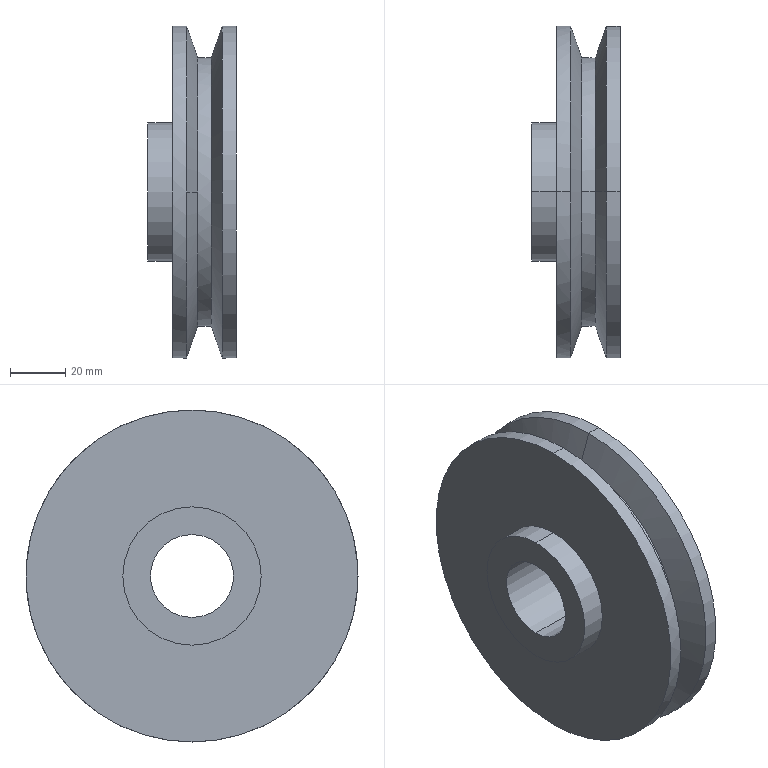Part | SolidWorks | features BaseBody 1, ICE 1 | 1 solid | 17 faces | box 32 x 120 x 120 mm | volume 219683 mm3 | cylinder 10 | cone 4 | plane 3 | commonest cylinder face diameters 120 x4 30 x2 50 x2 97.1 x2
STEP:
#1=CARTESIAN_POINT('',(21.,0.,-15.));
#2=VERTEX_POINT('',#1);
#3=CARTESIAN_POINT('',(21.,0.,15.));
#4=VERTEX_POINT('',#3);
#5=CARTESIAN_POINT('',(21.,0.,0.));
#6=DIRECTION('',(-1.,0.,0.));
#7=DIRECTION('',(0.,0.,1.));
#8=AXIS2_PLACEMENT_3D('',#5,#6,#7);
#9=CIRCLE('',#8,15.);
#10=EDGE_CURVE('',#2,#4,#9,.T.);
#11=ORIENTED_EDGE('',*,*,#10,.F.);
#12=CARTESIAN_POINT('',(-11.,0.,-15.));
#13=VERTEX_POINT('',#12);
#14=CARTESIAN_POINT('',(21.,0.,-15.));
#15=DIRECTION('',(-1.,0.,0.));
#16=VECTOR('',#15,1000.);
#17=LINE('',#14,#16);
#18=EDGE_CURVE('',#2,#13,#17,.T.);
#19=ORIENTED_EDGE('',*,*,#18,.T.);
#20=CARTESIAN_POINT('',(-11.,0.,15.));
#21=VERTEX_POINT('',#20);
#22=CARTESIAN_POINT('',(-11.,0.,0.));
#23=DIRECTION('',(-1.,0.,0.));
#24=DIRECTION('',(0.,0.,1.));
#25=AXIS2_PLACEMENT_3D('',#22,#23,#24);
#26=CIRCLE('',#25,15.);
#27=EDGE_CURVE('',#13,#21,#26,.T.);
#28=ORIENTED_EDGE('',*,*,#27,.T.);
#29=CARTESIAN_POINT('',(21.,0.,15.));
#30=DIRECTION('',(-1.,0.,0.));
#31=VECTOR('',#30,1000.);
#32=LINE('',#29,#31);
#33=EDGE_CURVE('',#4,#21,#32,.T.);
#34=ORIENTED_EDGE('',*,*,#33,.F.);
#35=EDGE_LOOP('',(#11,#19,#28,#34));
#36=FACE_OUTER_BOUND('',#35,.T.);
#37=CARTESIAN_POINT('',(21.,0.,0.));
#38=DIRECTION('',(-1.,0.,0.));
#39=DIRECTION('',(0.,0.,1.));
#40=AXIS2_PLACEMENT_3D('',#37,#38,#39);
#41=CYLINDRICAL_SURFACE('',#40,15.);
#42=ADVANCED_FACE('',(#36),#41,.F.);
#43=CARTESIAN_POINT('',(15.947,0.,-60.));
#44=VERTEX_POINT('',#43);
#45=CARTESIAN_POINT('',(15.947,0.,60.));
#46=VERTEX_POINT('',#45);
#47=CARTESIAN_POINT('',(15.947,0.,0.));
#48=DIRECTION('',(1.,0.,0.));
#49=DIRECTION('',(0.,0.,-1.));
#50=AXIS2_PLACEMENT_3D('',#47,#48,#49);
#51=CIRCLE('',#50,60.);
#52=EDGE_CURVE('',#44,#46,#51,.T.);
#53=ORIENTED_EDGE('',*,*,#52,.T.);
#54=CARTESIAN_POINT('',(21.,0.,60.));
#55=VERTEX_POINT('',#54);
#56=CARTESIAN_POINT('',(0.,0.,60.));
#57=DIRECTION('',(1.,0.,0.));
#58=VECTOR('',#57,1000.);
#59=LINE('',#56,#58);
#60=EDGE_CURVE('',#46,#55,#59,.T.);
#61=ORIENTED_EDGE('',*,*,#60,.T.);
#62=CARTESIAN_POINT('',(21.,0.,-60.));
#63=VERTEX_POINT('',#62);
#64=CARTESIAN_POINT('',(21.,0.,0.));
#65=DIRECTION('',(1.,0.,0.));
#66=DIRECTION('',(0.,0.,-1.));
#67=AXIS2_PLACEMENT_3D('',#64,#65,#66);
#68=CIRCLE('',#67,60.);
#69=EDGE_CURVE('',#63,#55,#68,.T.);
#70=ORIENTED_EDGE('',*,*,#69,.F.);
#71=CARTESIAN_POINT('',(0.,0.,-60.));
#72=DIRECTION('',(1.,0.,0.));
#73=VECTOR('',#72,1000.);
#74=LINE('',#71,#73);
#75=EDGE_CURVE('',#44,#63,#74,.T.);
#76=ORIENTED_EDGE('',*,*,#75,.F.);
#77=EDGE_LOOP('',(#53,#61,#70,#76));
#78=FACE_OUTER_BOUND('',#77,.T.);
#79=CARTESIAN_POINT('',(0.,0.,0.));
#80=DIRECTION('',(1.,0.,0.));
#81=DIRECTION('',(0.,0.,-1.));
#82=AXIS2_PLACEMENT_3D('',#79,#80,#81);
#83=CYLINDRICAL_SURFACE('',#82,60.);
#84=ADVANCED_FACE('',(#78),#83,.T.);
#85=CARTESIAN_POINT('',(12.004,0.,-48.55));
#86=VERTEX_POINT('',#85);
#87=CARTESIAN_POINT('',(12.004,0.,48.55));
#88=VERTEX_POINT('',#87);
#89=CARTESIAN_POINT('',(12.004,0.,0.));
#90=DIRECTION('',(1.,0.,0.));
#91=DIRECTION('',(0.,0.,-1.));
#92=AXIS2_PLACEMENT_3D('',#89,#90,#91);
#93=CIRCLE('',#92,48.55);
#94=EDGE_CURVE('',#86,#88,#93,.T.);
#95=ORIENTED_EDGE('',*,*,#94,.T.);
#96=CARTESIAN_POINT('',(15.947,0.,60.));
#97=DIRECTION('',(0.3256,0.,0.9455));
#98=VECTOR('',#97,1000.);
#99=LINE('',#96,#98);
#100=EDGE_CURVE('',#88,#46,#99,.T.);
#101=ORIENTED_EDGE('',*,*,#100,.T.);
#102=ORIENTED_EDGE('',*,*,#52,.F.);
#103=CARTESIAN_POINT('',(15.947,0.,-60.));
#104=DIRECTION('',(0.3256,0.,-0.9455));
#105=VECTOR('',#104,1000.);
#106=LINE('',#103,#105);
#107=EDGE_CURVE('',#86,#44,#106,.T.);
#108=ORIENTED_EDGE('',*,*,#107,.F.);
#109=EDGE_LOOP('',(#95,#101,#102,#108));
#110=FACE_OUTER_BOUND('',#109,.T.);
#111=CARTESIAN_POINT('',(15.947,0.,0.));
#112=DIRECTION('',(1.,0.,0.));
#113=DIRECTION('',(0.,0.,-1.));
#114=AXIS2_PLACEMENT_3D('',#111,#112,#113);
#115=CONICAL_SURFACE('',#114,60.,1.239);
#116=ADVANCED_FACE('',(#110),#115,.T.);
#117=CARTESIAN_POINT('',(-11.,0.,25.));
#118=VERTEX_POINT('',#117);
#119=CARTESIAN_POINT('',(-11.,0.,-25.));
#120=VERTEX_POINT('',#119);
#121=CARTESIAN_POINT('',(-11.,0.,0.));
#122=DIRECTION('',(-1.,0.,0.));
#123=DIRECTION('',(0.,0.,-1.));
#124=AXIS2_PLACEMENT_3D('',#121,#122,#123);
#125=CIRCLE('',#124,25.);
#126=EDGE_CURVE('',#118,#120,#125,.T.);
#127=ORIENTED_EDGE('',*,*,#126,.F.);
#128=CARTESIAN_POINT('',(-2.,0.,25.));
#129=VERTEX_POINT('',#128);
#130=CARTESIAN_POINT('',(0.,0.,25.));
#131=DIRECTION('',(1.,0.,0.));
#132=VECTOR('',#131,1000.);
#133=LINE('',#130,#132);
#134=EDGE_CURVE('',#118,#129,#133,.T.);
#135=ORIENTED_EDGE('',*,*,#134,.T.);
#136=CARTESIAN_POINT('',(-2.,0.,-25.));
#137=VERTEX_POINT('',#136);
#138=CARTESIAN_POINT('',(-2.,0.,0.));
#139=DIRECTION('',(-1.,0.,0.));
#140=DIRECTION('',(0.,0.,-1.));
#141=AXIS2_PLACEMENT_3D('',#138,#139,#140);
#142=CIRCLE('',#141,25.);
#143=EDGE_CURVE('',#129,#137,#142,.T.);
#144=ORIENTED_EDGE('',*,*,#143,.T.);
#145=CARTESIAN_POINT('',(0.,0.,-25.));
#146=DIRECTION('',(1.,0.,0.));
#147=VECTOR('',#146,1000.);
#148=LINE('',#145,#147);
#149=EDGE_CURVE('',#120,#137,#148,.T.);
#150=ORIENTED_EDGE('',*,*,#149,.F.);
#151=EDGE_LOOP('',(#127,#135,#144,#150));
#152=FACE_OUTER_BOUND('',#151,.T.);
#153=CARTESIAN_POINT('',(0.,0.,0.));
#154=DIRECTION('',(1.,0.,0.));
#155=DIRECTION('',(0.,0.,-1.));
#156=AXIS2_PLACEMENT_3D('',#153,#154,#155);
#157=CYLINDRICAL_SURFACE('',#156,25.);
#158=ADVANCED_FACE('',(#152),#157,.T.);
#159=ORIENTED_EDGE('',*,*,#94,.F.);
#160=CARTESIAN_POINT('',(6.996,0.,-48.55));
#161=VERTEX_POINT('',#160);
#162=CARTESIAN_POINT('',(0.,0.,-48.55));
#163=DIRECTION('',(-1.,0.,0.));
#164=VECTOR('',#163,1000.);
#165=LINE('',#162,#164);
#166=EDGE_CURVE('',#86,#161,#165,.T.);
#167=ORIENTED_EDGE('',*,*,#166,.T.);
#168=CARTESIAN_POINT('',(6.996,48.55,0.));
#169=VERTEX_POINT('',#168);
#170=CARTESIAN_POINT('',(6.996,0.,0.));
#171=DIRECTION('',(1.,0.,0.));
#172=DIRECTION('',(0.,0.,1.));
#173=AXIS2_PLACEMENT_3D('',#170,#171,#172);
#174=CIRCLE('',#173,48.55);
#175=EDGE_CURVE('',#161,#169,#174,.T.);
#176=ORIENTED_EDGE('',*,*,#175,.T.);
#177=CARTESIAN_POINT('',(6.996,0.,48.55));
#178=VERTEX_POINT('',#177);
#179=CARTESIAN_POINT('',(6.996,0.,0.));
#180=DIRECTION('',(1.,0.,0.));
#181=DIRECTION('',(0.,0.,1.));
#182=AXIS2_PLACEMENT_3D('',#179,#180,#181);
#183=CIRCLE('',#182,48.55);
#184=EDGE_CURVE('',#169,#178,#183,.T.);
#185=ORIENTED_EDGE('',*,*,#184,.T.);
#186=CARTESIAN_POINT('',(0.,0.,48.55));
#187=DIRECTION('',(-1.,0.,0.));
#188=VECTOR('',#187,1000.);
#189=LINE('',#186,#188);
#190=EDGE_CURVE('',#88,#178,#189,.T.);
#191=ORIENTED_EDGE('',*,*,#190,.F.);
#192=EDGE_LOOP('',(#159,#167,#176,#185,#191));
#193=FACE_OUTER_BOUND('',#192,.T.);
#194=CARTESIAN_POINT('',(0.,0.,0.));
#195=DIRECTION('',(-1.,0.,0.));
#196=DIRECTION('',(0.,0.,1.));
#197=AXIS2_PLACEMENT_3D('',#194,#195,#196);
#198=CYLINDRICAL_SURFACE('',#197,48.55);
#199=ADVANCED_FACE('',(#193),#198,.T.);
#200=ORIENTED_EDGE('',*,*,#184,.F.);
#201=CARTESIAN_POINT('',(3.053,60.,0.));
#202=VERTEX_POINT('',#201);
#203=CARTESIAN_POINT('',(3.053,60.,0.));
#204=DIRECTION('',(-0.3256,0.9455,0.));
#205=VECTOR('',#204,1000.);
#206=LINE('',#203,#205);
#207=EDGE_CURVE('',#169,#202,#206,.T.);
#208=ORIENTED_EDGE('',*,*,#207,.T.);
#209=CARTESIAN_POINT('',(3.053,0.,60.));
#210=VERTEX_POINT('',#209);
#211=CARTESIAN_POINT('',(3.053,0.,0.));
#212=DIRECTION('',(1.,0.,0.));
#213=DIRECTION('',(0.,0.,1.));
#214=AXIS2_PLACEMENT_3D('',#211,#212,#213);
#215=CIRCLE('',#214,60.);
#216=EDGE_CURVE('',#202,#210,#215,.T.);
#217=ORIENTED_EDGE('',*,*,#216,.T.);
#218=CARTESIAN_POINT('',(3.053,-60.,0.));
#219=VERTEX_POINT('',#218);
#220=CARTESIAN_POINT('',(3.053,0.,0.));
#221=DIRECTION('',(1.,0.,0.));
#222=DIRECTION('',(0.,0.,1.));
#223=AXIS2_PLACEMENT_3D('',#220,#221,#222);
#224=CIRCLE('',#223,60.);
#225=EDGE_CURVE('',#210,#219,#224,.T.);
#226=ORIENTED_EDGE('',*,*,#225,.T.);
#227=CARTESIAN_POINT('',(6.996,-48.55,0.));
#228=VERTEX_POINT('',#227);
#229=CARTESIAN_POINT('',(3.053,-60.,0.));
#230=DIRECTION('',(-0.3256,-0.9455,0.));
#231=VECTOR('',#230,1000.);
#232=LINE('',#229,#231);
#233=EDGE_CURVE('',#228,#219,#232,.T.);
#234=ORIENTED_EDGE('',*,*,#233,.F.);
#235=CARTESIAN_POINT('',(6.996,0.,0.));
#236=DIRECTION('',(1.,0.,0.));
#237=DIRECTION('',(0.,0.,1.));
#238=AXIS2_PLACEMENT_3D('',#235,#236,#237);
#239=CIRCLE('',#238,48.55);
#240=EDGE_CURVE('',#178,#228,#239,.T.);
#241=ORIENTED_EDGE('',*,*,#240,.F.);
#242=EDGE_LOOP('',(#200,#208,#217,#226,#234,#241));
#243=FACE_OUTER_BOUND('',#242,.T.);
#244=CARTESIAN_POINT('',(3.053,0.,0.));
#245=DIRECTION('',(-1.,0.,0.));
#246=DIRECTION('',(0.,-1.,0.));
#247=AXIS2_PLACEMENT_3D('',#244,#245,#246);
#248=CONICAL_SURFACE('',#247,60.,1.239);
#249=ADVANCED_FACE('',(#243),#248,.T.);
#250=CARTESIAN_POINT('',(-2.,0.,60.));
#251=VERTEX_POINT('',#250);
#252=CARTESIAN_POINT('',(-2.,0.,-60.));
#253=VERTEX_POINT('',#252);
#254=CARTESIAN_POINT('',(-2.,0.,0.));
#255=DIRECTION('',(-1.,0.,0.));
#256=DIRECTION('',(0.,0.,-1.));
#257=AXIS2_PLACEMENT_3D('',#254,#255,#256);
#258=CIRCLE('',#257,60.);
#259=EDGE_CURVE('',#251,#253,#258,.T.);
#260=ORIENTED_EDGE('',*,*,#259,.F.);
#261=CARTESIAN_POINT('',(0.,0.,60.));
#262=DIRECTION('',(1.,0.,0.));
#263=VECTOR('',#262,1000.);
#264=LINE('',#261,#263);
#265=EDGE_CURVE('',#251,#210,#264,.T.);
#266=ORIENTED_EDGE('',*,*,#265,.T.);
#267=ORIENTED_EDGE('',*,*,#216,.F.);
#268=CARTESIAN_POINT('',(3.053,0.,-60.));
#269=VERTEX_POINT('',#268);
#270=CARTESIAN_POINT('',(3.053,0.,0.));
#271=DIRECTION('',(1.,0.,0.));
#272=DIRECTION('',(0.,0.,1.));
#273=AXIS2_PLACEMENT_3D('',#270,#271,#272);
#274=CIRCLE('',#273,60.);
#275=EDGE_CURVE('',#269,#202,#274,.T.);
#276=ORIENTED_EDGE('',*,*,#275,.F.);
#277=CARTESIAN_POINT('',(0.,0.,-60.));
#278=DIRECTION('',(1.,0.,0.));
#279=VECTOR('',#278,1000.);
#280=LINE('',#277,#279);
#281=EDGE_CURVE('',#253,#269,#280,.T.);
#282=ORIENTED_EDGE('',*,*,#281,.F.);
#283=EDGE_LOOP('',(#260,#266,#267,#276,#282));
#284=FACE_OUTER_BOUND('',#283,.T.);
#285=CARTESIAN_POINT('',(0.,0.,0.));
#286=DIRECTION('',(1.,0.,0.));
#287=DIRECTION('',(0.,0.,-1.));
#288=AXIS2_PLACEMENT_3D('',#285,#286,#287);
#289=CYLINDRICAL_SURFACE('',#288,60.);
#290=ADVANCED_FACE('',(#284),#289,.T.);
#291=CARTESIAN_POINT('',(21.,0.,0.));
#292=DIRECTION('',(-1.,0.,0.));
#293=DIRECTION('',(0.,0.,1.));
#294=AXIS2_PLACEMENT_3D('',#291,#292,#293);
#295=CIRCLE('',#294,15.);
#296=EDGE_CURVE('',#4,#2,#295,.T.);
#297=ORIENTED_EDGE('',*,*,#296,.T.);
#298=ORIENTED_EDGE('',*,*,#10,.T.);
#299=EDGE_LOOP('',(#297,#298));
#300=FACE_BOUND('',#299,.T.);
#301=ORIENTED_EDGE('',*,*,#69,.T.);
#302=CARTESIAN_POINT('',(21.,0.,0.));
#303=DIRECTION('',(1.,0.,0.));
#304=DIRECTION('',(0.,0.,-1.));
#305=AXIS2_PLACEMENT_3D('',#302,#303,#304);
#306=CIRCLE('',#305,60.);
#307=EDGE_CURVE('',#55,#63,#306,.T.);
#308=ORIENTED_EDGE('',*,*,#307,.T.);
#309=EDGE_LOOP('',(#301,#308));
#310=FACE_OUTER_BOUND('',#309,.T.);
#311=CARTESIAN_POINT('',(21.,60.,0.));
#312=DIRECTION('',(1.,0.,0.));
#313=DIRECTION('',(0.,0.,-1.));
#314=AXIS2_PLACEMENT_3D('',#311,#312,#313);
#315=PLANE('',#314);
#316=ADVANCED_FACE('',(#300,#310),#315,.T.);
#317=ORIENTED_EDGE('',*,*,#60,.F.);
#318=CARTESIAN_POINT('',(15.947,0.,0.));
#319=DIRECTION('',(1.,0.,0.));
#320=DIRECTION('',(0.,0.,-1.));
#321=AXIS2_PLACEMENT_3D('',#318,#319,#320);
#322=CIRCLE('',#321,60.);
#323=EDGE_CURVE('',#46,#44,#322,.T.);
#324=ORIENTED_EDGE('',*,*,#323,.T.);
#325=ORIENTED_EDGE('',*,*,#75,.T.);
#326=ORIENTED_EDGE('',*,*,#307,.F.);
#327=EDGE_LOOP('',(#317,#324,#325,#326));
#328=FACE_OUTER_BOUND('',#327,.T.);
#329=CARTESIAN_POINT('',(0.,0.,0.));
#330=DIRECTION('',(1.,0.,0.));
#331=DIRECTION('',(0.,0.,-1.));
#332=AXIS2_PLACEMENT_3D('',#329,#330,#331);
#333=CYLINDRICAL_SURFACE('',#332,60.);
#334=ADVANCED_FACE('',(#328),#333,.T.);
#335=CARTESIAN_POINT('',(-11.,0.,0.));
#336=DIRECTION('',(-1.,0.,0.));
#337=DIRECTION('',(0.,0.,1.));
#338=AXIS2_PLACEMENT_3D('',#335,#336,#337);
#339=CIRCLE('',#338,15.);
#340=EDGE_CURVE('',#21,#13,#339,.T.);
#341=ORIENTED_EDGE('',*,*,#340,.F.);
#342=ORIENTED_EDGE('',*,*,#27,.F.);
#343=EDGE_LOOP('',(#341,#342));
#344=FACE_BOUND('',#343,.T.);
#345=CARTESIAN_POINT('',(-11.,0.,0.));
#346=DIRECTION('',(-1.,0.,0.));
#347=DIRECTION('',(0.,0.,-1.));
#348=AXIS2_PLACEMENT_3D('',#345,#346,#347);
#349=CIRCLE('',#348,25.);
#350=EDGE_CURVE('',#120,#118,#349,.T.);
#351=ORIENTED_EDGE('',*,*,#350,.T.);
#352=ORIENTED_EDGE('',*,*,#126,.T.);
#353=EDGE_LOOP('',(#351,#352));
#354=FACE_OUTER_BOUND('',#353,.T.);
#355=CARTESIAN_POINT('',(-11.,0.,0.));
#356=DIRECTION('',(-1.,0.,0.));
#357=DIRECTION('',(0.,0.,1.));
#358=AXIS2_PLACEMENT_3D('',#355,#356,#357);
#359=PLANE('',#358);
#360=ADVANCED_FACE('',(#344,#354),#359,.T.);
#361=ORIENTED_EDGE('',*,*,#100,.F.);
#362=CARTESIAN_POINT('',(12.004,0.,0.));
#363=DIRECTION('',(1.,0.,0.));
#364=DIRECTION('',(0.,0.,-1.));
#365=AXIS2_PLACEMENT_3D('',#362,#363,#364);
#366=CIRCLE('',#365,48.55);
#367=EDGE_CURVE('',#88,#86,#366,.T.);
#368=ORIENTED_EDGE('',*,*,#367,.T.);
#369=ORIENTED_EDGE('',*,*,#107,.T.);
#370=ORIENTED_EDGE('',*,*,#323,.F.);
#371=EDGE_LOOP('',(#361,#368,#369,#370));
#372=FACE_OUTER_BOUND('',#371,.T.);
#373=CARTESIAN_POINT('',(15.947,0.,0.));
#374=DIRECTION('',(1.,0.,0.));
#375=DIRECTION('',(0.,0.,-1.));
#376=AXIS2_PLACEMENT_3D('',#373,#374,#375);
#377=CONICAL_SURFACE('',#376,60.,1.239);
#378=ADVANCED_FACE('',(#372),#377,.T.);
#379=ORIENTED_EDGE('',*,*,#134,.F.);
#380=ORIENTED_EDGE('',*,*,#350,.F.);
#381=ORIENTED_EDGE('',*,*,#149,.T.);
#382=CARTESIAN_POINT('',(-2.,0.,0.));
#383=DIRECTION('',(-1.,0.,0.));
#384=DIRECTION('',(0.,0.,-1.));
#385=AXIS2_PLACEMENT_3D('',#382,#383,#384);
#386=CIRCLE('',#385,25.);
#387=EDGE_CURVE('',#137,#129,#386,.T.);
#388=ORIENTED_EDGE('',*,*,#387,.T.);
#389=EDGE_LOOP('',(#379,#380,#381,#388));
#390=FACE_OUTER_BOUND('',#389,.T.);
#391=CARTESIAN_POINT('',(0.,0.,0.));
#392=DIRECTION('',(1.,0.,0.));
#393=DIRECTION('',(0.,0.,-1.));
#394=AXIS2_PLACEMENT_3D('',#391,#392,#393);
#395=CYLINDRICAL_SURFACE('',#394,25.);
#396=ADVANCED_FACE('',(#390),#395,.T.);
#397=ORIENTED_EDGE('',*,*,#166,.F.);
#398=ORIENTED_EDGE('',*,*,#367,.F.);
#399=ORIENTED_EDGE('',*,*,#190,.T.);
#400=ORIENTED_EDGE('',*,*,#240,.T.);
#401=CARTESIAN_POINT('',(6.996,0.,0.));
#402=DIRECTION('',(1.,0.,0.));
#403=DIRECTION('',(0.,0.,1.));
#404=AXIS2_PLACEMENT_3D('',#401,#402,#403);
#405=CIRCLE('',#404,48.55);
#406=EDGE_CURVE('',#228,#161,#405,.T.);
#407=ORIENTED_EDGE('',*,*,#406,.T.);
#408=EDGE_LOOP('',(#397,#398,#399,#400,#407));
#409=FACE_OUTER_BOUND('',#408,.T.);
#410=CARTESIAN_POINT('',(0.,0.,0.));
#411=DIRECTION('',(-1.,0.,0.));
#412=DIRECTION('',(0.,0.,1.));
#413=AXIS2_PLACEMENT_3D('',#410,#411,#412);
#414=CYLINDRICAL_SURFACE('',#413,48.55);
#415=ADVANCED_FACE('',(#409),#414,.T.);
#416=CARTESIAN_POINT('',(-2.,0.,0.));
#417=DIRECTION('',(-1.,0.,0.));
#418=DIRECTION('',(0.,0.,-1.));
#419=AXIS2_PLACEMENT_3D('',#416,#417,#418);
#420=CIRCLE('',#419,60.);
#421=EDGE_CURVE('',#253,#251,#420,.T.);
#422=ORIENTED_EDGE('',*,*,#421,.T.);
#423=ORIENTED_EDGE('',*,*,#259,.T.);
#424=EDGE_LOOP('',(#422,#423));
#425=FACE_OUTER_BOUND('',#424,.T.);
#426=ORIENTED_EDGE('',*,*,#387,.F.);
#427=ORIENTED_EDGE('',*,*,#143,.F.);
#428=EDGE_LOOP('',(#426,#427));
#429=FACE_BOUND('',#428,.T.);
#430=CARTESIAN_POINT('',(-2.,60.,0.));
#431=DIRECTION('',(-1.,0.,0.));
#432=DIRECTION('',(0.,0.,1.));
#433=AXIS2_PLACEMENT_3D('',#430,#431,#432);
#434=PLANE('',#433);
#435=ADVANCED_FACE('',(#425,#429),#434,.T.);
#436=ORIENTED_EDGE('',*,*,#207,.F.);
#437=ORIENTED_EDGE('',*,*,#175,.F.);
#438=ORIENTED_EDGE('',*,*,#406,.F.);
#439=ORIENTED_EDGE('',*,*,#233,.T.);
#440=CARTESIAN_POINT('',(3.053,0.,0.));
#441=DIRECTION('',(1.,0.,0.));
#442=DIRECTION('',(0.,0.,1.));
#443=AXIS2_PLACEMENT_3D('',#440,#441,#442);
#444=CIRCLE('',#443,60.);
#445=EDGE_CURVE('',#219,#269,#444,.T.);
#446=ORIENTED_EDGE('',*,*,#445,.T.);
#447=ORIENTED_EDGE('',*,*,#275,.T.);
#448=EDGE_LOOP('',(#436,#437,#438,#439,#446,#447));
#449=FACE_OUTER_BOUND('',#448,.T.);
#450=CARTESIAN_POINT('',(3.053,0.,0.));
#451=DIRECTION('',(-1.,0.,0.));
#452=DIRECTION('',(0.,-1.,0.));
#453=AXIS2_PLACEMENT_3D('',#450,#451,#452);
#454=CONICAL_SURFACE('',#453,60.,1.239);
#455=ADVANCED_FACE('',(#449),#454,.T.);
#456=ORIENTED_EDGE('',*,*,#265,.F.);
#457=ORIENTED_EDGE('',*,*,#421,.F.);
#458=ORIENTED_EDGE('',*,*,#281,.T.);
#459=ORIENTED_EDGE('',*,*,#445,.F.);
#460=ORIENTED_EDGE('',*,*,#225,.F.);
#461=EDGE_LOOP('',(#456,#457,#458,#459,#460));
#462=FACE_OUTER_BOUND('',#461,.T.);
#463=CARTESIAN_POINT('',(0.,0.,0.));
#464=DIRECTION('',(1.,0.,0.));
#465=DIRECTION('',(0.,0.,-1.));
#466=AXIS2_PLACEMENT_3D('',#463,#464,#465);
#467=CYLINDRICAL_SURFACE('',#466,60.);
#468=ADVANCED_FACE('',(#462),#467,.T.);
#469=ORIENTED_EDGE('',*,*,#18,.F.);
#470=ORIENTED_EDGE('',*,*,#296,.F.);
#471=ORIENTED_EDGE('',*,*,#33,.T.);
#472=ORIENTED_EDGE('',*,*,#340,.T.);
#473=EDGE_LOOP('',(#469,#470,#471,#472));
#474=FACE_OUTER_BOUND('',#473,.T.);
#475=CARTESIAN_POINT('',(21.,0.,0.));
#476=DIRECTION('',(-1.,0.,0.));
#477=DIRECTION('',(0.,0.,1.));
#478=AXIS2_PLACEMENT_3D('',#475,#476,#477);
#479=CYLINDRICAL_SURFACE('',#478,15.);
#480=ADVANCED_FACE('',(#474),#479,.F.);
#481=CLOSED_SHELL('',(#42,#84,#116,#158,#199,#249,#290,#316,#334,#360,#378,#396,#415,#435,#455,#468,#480));
#482=MANIFOLD_SOLID_BREP('',#481);
#483=CARTESIAN_POINT('',(0.,0.,0.));
#484=DIRECTION('',(0.,0.,1.));
#485=DIRECTION('',(1.,0.,0.));
#486=AXIS2_PLACEMENT_3D('',#483,#484,#485);
#487=(LENGTH_UNIT()NAMED_UNIT(*)SI_UNIT(.MILLI.,.METRE.));
#488=UNCERTAINTY_MEASURE_WITH_UNIT(LENGTH_MEASURE(0.00001),#487,'','');
#489=(NAMED_UNIT(*)PLANE_ANGLE_UNIT()SI_UNIT($,.RADIAN.));
#490=(NAMED_UNIT(*)SI_UNIT($,.STERADIAN.)SOLID_ANGLE_UNIT());
#491=(GEOMETRIC_REPRESENTATION_CONTEXT(3)GLOBAL_UNCERTAINTY_ASSIGNED_CONTEXT((#488))GLOBAL_UNIT_ASSIGNED_CONTEXT((#487,#489,#490))REPRESENTATION_CONTEXT('',''));
#492=ADVANCED_BREP_SHAPE_REPRESENTATION('',(#482,#486),#491);